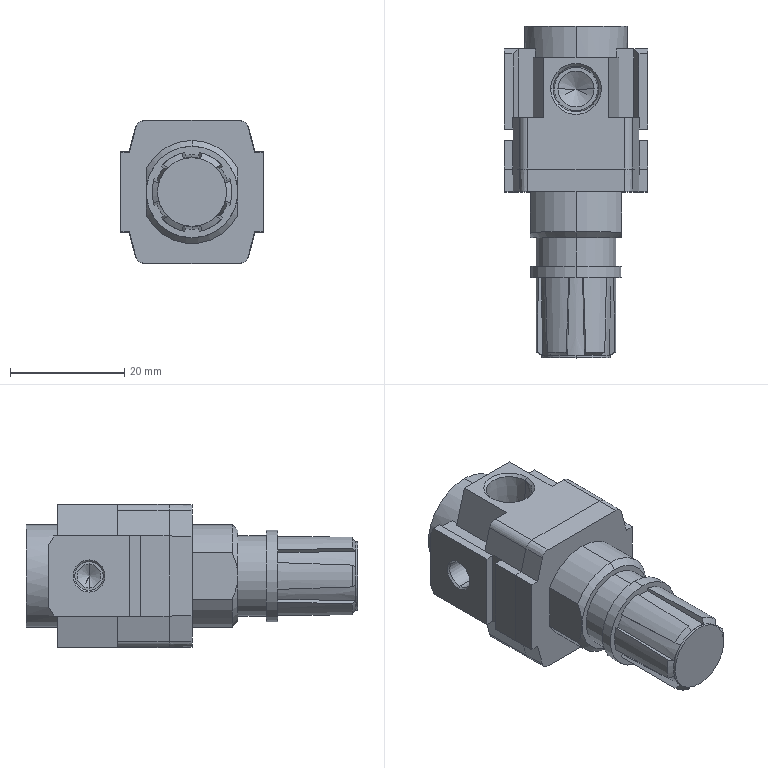Part | STEP file | AC10B-M5_AC3011A AR Body(10)-1 | 1 solid | 156 faces | box 25 x 58 x 25 mm | volume 17859 mm3 | plane 88 | cone 35 | cylinder 33 | commonest cylinder face diameters 14 x8 18 x5 3 x4 4.2 x4 5 x4 6.3 x4